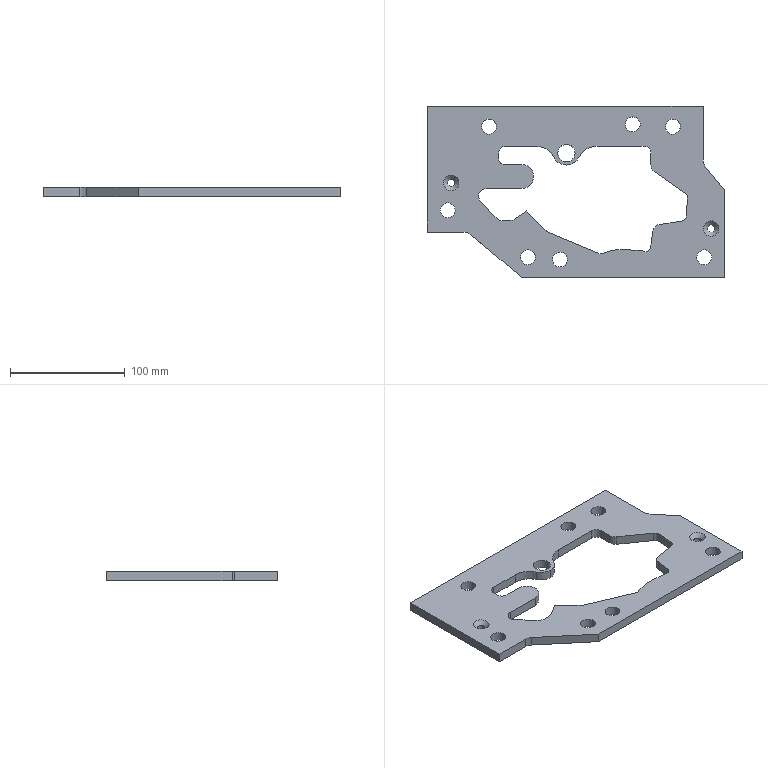Part | STEP file | gslz 2016.10.28-13_id130_x_t | 1 solid | 63 faces | box 260 x 150 x 8 mm | volume 185051 mm3 | cylinder 32 | plane 29 | cone 2 | commonest cylinder face diameters 10 x8 13 x7 12 x3 6.5 x2 14 x2 18 x2